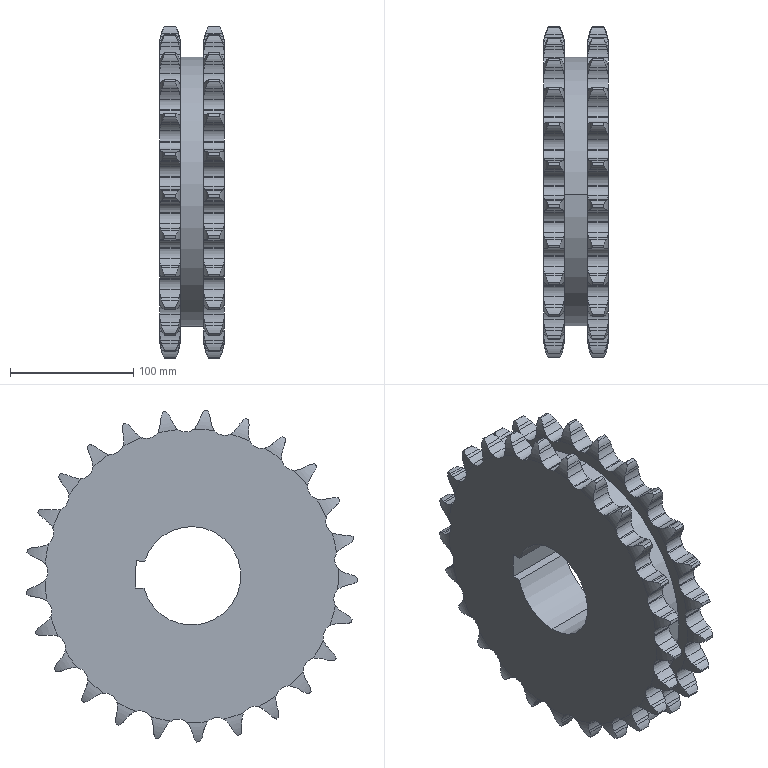Part | STEP file | Input 74 | 1 solid | 640 faces | box 52.8 x 269.775 x 269.908 mm | volume 2050687 mm3 | cylinder 379 | plane 157 | torus 104 | commonest cylinder face diameters 19.221 x114 31.288 x106 49.701 x104 270.377 x50 80 x3 218.815 x2